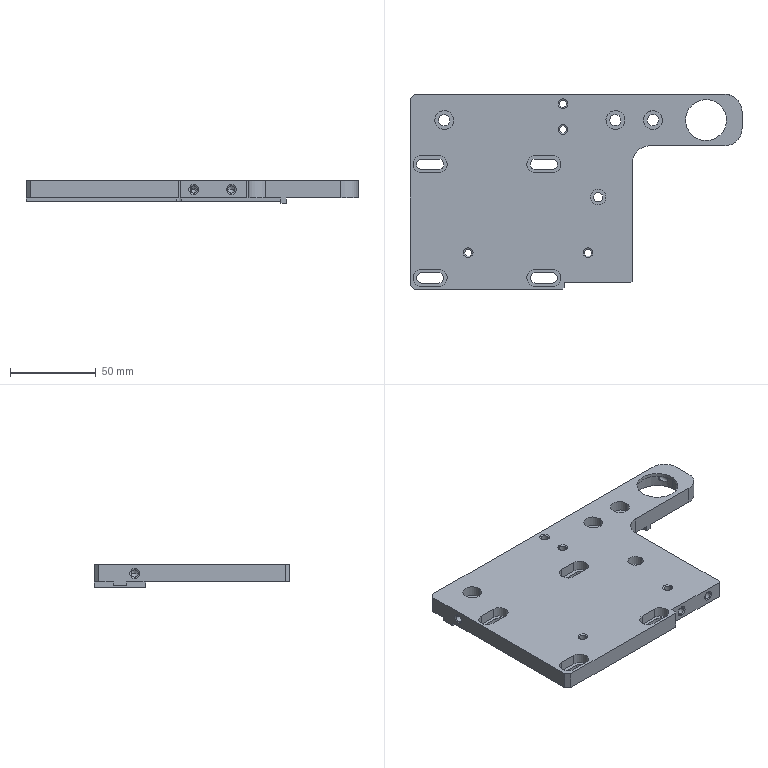Part | STEP file | 11-SS103_PRT_BODY_1-1.PRT11 | 1 solid | 143 faces | box 194 x 114 x 13 mm | volume 152275 mm3 | cylinder 68 | plane 48 | cone 27 | commonest cylinder face diameters 4.2 x21 3.3 x8 6 x8 10 x8 6.6 x6 11 x6